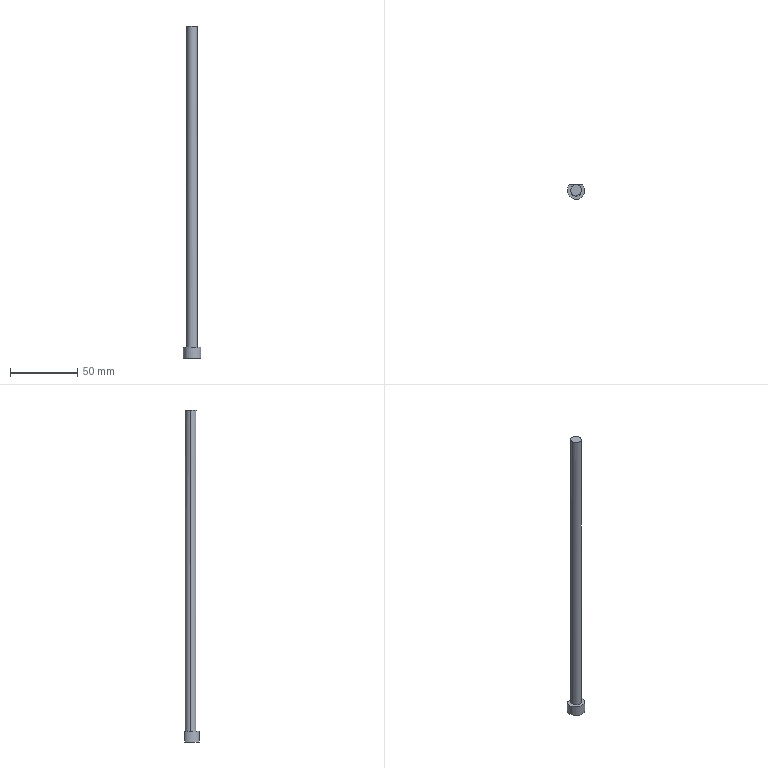Part | Creo | 1 solid | 7 faces | box 13 x 11 x 246.801 mm | volume 12961 mm3 | plane 4 | cylinder 3 | commonest cylinder face diameters 8 x2 13 x1
STEP:
#1=CARTESIAN_POINT('',(0.,0.,0.));
#2=DIRECTION('',(0.,0.,1.));
#3=DIRECTION('',(1.,0.,0.));
#4=AXIS2_PLACEMENT_3D('',#1,#2,#3);
#5=CARTESIAN_POINT('',(94.951,-2.288,-330.441));
#6=VERTEX_POINT('',#5);
#7=CARTESIAN_POINT('',(93.142,-6.788,-330.441));
#8=VERTEX_POINT('',#7);
#9=CARTESIAN_POINT('',(99.642,-6.788,-330.441));
#10=DIRECTION('',(0.,0.,1.));
#11=DIRECTION('',(-0.7216,0.6923,0.));
#12=AXIS2_PLACEMENT_3D('',#9,#10,#11);
#13=CIRCLE('',#12,6.5);
#14=EDGE_CURVE('',#6,#8,#13,.T.);
#15=ORIENTED_EDGE('',*,*,#14,.F.);
#16=CARTESIAN_POINT('',(104.332,-2.288,-330.441));
#17=VERTEX_POINT('',#16);
#18=CARTESIAN_POINT('',(94.951,-2.288,-330.441));
#19=DIRECTION('',(1.,0.,0.));
#20=VECTOR('',#19,9.381);
#21=LINE('',#18,#20);
#22=EDGE_CURVE('',#6,#17,#21,.T.);
#23=ORIENTED_EDGE('',*,*,#22,.T.);
#24=CARTESIAN_POINT('',(99.642,-6.788,-330.441));
#25=DIRECTION('',(0.,0.,1.));
#26=DIRECTION('',(-1.,0.,0.));
#27=AXIS2_PLACEMENT_3D('',#24,#25,#26);
#28=CIRCLE('',#27,6.5);
#29=EDGE_CURVE('',#8,#17,#28,.T.);
#30=ORIENTED_EDGE('',*,*,#29,.F.);
#31=EDGE_LOOP('',(#15,#23,#30));
#32=FACE_OUTER_BOUND('',#31,.F.);
#33=CARTESIAN_POINT('',(103.642,-6.788,-330.441));
#34=VERTEX_POINT('',#33);
#35=CARTESIAN_POINT('',(95.642,-6.788,-330.441));
#36=VERTEX_POINT('',#35);
#37=CARTESIAN_POINT('',(99.642,-6.788,-330.441));
#38=DIRECTION('',(0.,0.,-1.));
#39=DIRECTION('',(1.,0.,0.));
#40=AXIS2_PLACEMENT_3D('',#37,#38,#39);
#41=CIRCLE('',#40,4.);
#42=EDGE_CURVE('',#34,#36,#41,.T.);
#43=ORIENTED_EDGE('',*,*,#42,.F.);
#44=CARTESIAN_POINT('',(99.642,-6.788,-330.441));
#45=DIRECTION('',(0.,0.,-1.));
#46=DIRECTION('',(-1.,0.,0.));
#47=AXIS2_PLACEMENT_3D('',#44,#45,#46);
#48=CIRCLE('',#47,4.);
#49=EDGE_CURVE('',#36,#34,#48,.T.);
#50=ORIENTED_EDGE('',*,*,#49,.F.);
#51=EDGE_LOOP('',(#43,#50));
#52=FACE_BOUND('',#51,.F.);
#53=CARTESIAN_POINT('',(99.642,-6.788,-330.441));
#54=DIRECTION('',(0.,0.,1.));
#55=DIRECTION('',(1.,0.,0.));
#56=AXIS2_PLACEMENT_3D('',#53,#54,#55);
#57=PLANE('',#56);
#58=ADVANCED_FACE('',(#32,#52),#57,.T.);
#59=ORIENTED_EDGE('',*,*,#42,.T.);
#60=CARTESIAN_POINT('',(95.642,-6.786,-91.64));
#61=VERTEX_POINT('',#60);
#62=CARTESIAN_POINT('',(95.642,-6.788,-330.441));
#63=DIRECTION('',(0.000000004,0.000007085,1.));
#64=VECTOR('',#63,238.801);
#65=LINE('',#62,#64);
#66=EDGE_CURVE('',#36,#61,#65,.T.);
#67=ORIENTED_EDGE('',*,*,#66,.T.);
#68=CARTESIAN_POINT('',(103.642,-6.788,-91.651));
#69=VERTEX_POINT('',#68);
#70=CARTESIAN_POINT('',(95.642,-6.786,-91.64));
#71=CARTESIAN_POINT('',(95.642,-7.182,-91.64));
#72=CARTESIAN_POINT('',(95.752,-7.93,-91.641));
#73=CARTESIAN_POINT('',(96.234,-8.986,-91.641));
#74=CARTESIAN_POINT('',(96.983,-9.847,-91.642));
#75=CARTESIAN_POINT('',(97.943,-10.47,-91.643));
#76=CARTESIAN_POINT('',(99.052,-10.8,-91.645));
#77=CARTESIAN_POINT('',(100.2,-10.804,-91.646));
#78=CARTESIAN_POINT('',(101.309,-10.484,-91.648));
#79=CARTESIAN_POINT('',(102.279,-9.867,-91.649));
#80=CARTESIAN_POINT('',(103.042,-9.001,-91.65));
#81=CARTESIAN_POINT('',(103.531,-7.934,-91.651));
#82=CARTESIAN_POINT('',(103.642,-7.182,-91.651));
#83=CARTESIAN_POINT('',(103.642,-6.788,-91.651));
#84=B_SPLINE_CURVE_WITH_KNOTS('',3,(#70,#71,#72,#73,#74,#75,#76,#77,#78,#79,#80,#81,#82,#83),.UNSPECIFIED.,.F.,.F.,(4,1,1,1,1,1,1,1,1,1,1,4),(0.,0.09091,0.1818,0.2727,0.3636,0.4545,0.5455,0.6364,0.7273,0.8182,0.9091,1.),.UNSPECIFIED.);
#85=EDGE_CURVE('',#61,#69,#84,.T.);
#86=ORIENTED_EDGE('',*,*,#85,.T.);
#87=CARTESIAN_POINT('',(103.642,-6.788,-330.441));
#88=DIRECTION('',(0.,0.,1.));
#89=VECTOR('',#88,238.791);
#90=LINE('',#87,#89);
#91=EDGE_CURVE('',#34,#69,#90,.T.);
#92=ORIENTED_EDGE('',*,*,#91,.F.);
#93=EDGE_LOOP('',(#59,#67,#86,#92));
#94=FACE_OUTER_BOUND('',#93,.F.);
#95=CARTESIAN_POINT('',(99.642,-6.788,-653.441));
#96=DIRECTION('',(0.,0.,1.));
#97=DIRECTION('',(1.,0.,0.));
#98=AXIS2_PLACEMENT_3D('',#95,#96,#97);
#99=CYLINDRICAL_SURFACE('',#98,4.);
#100=ADVANCED_FACE('',(#94),#99,.T.);
#101=ORIENTED_EDGE('',*,*,#49,.T.);
#102=ORIENTED_EDGE('',*,*,#91,.T.);
#103=CARTESIAN_POINT('',(103.642,-6.788,-91.651));
#104=CARTESIAN_POINT('',(103.642,-6.395,-91.651));
#105=CARTESIAN_POINT('',(103.531,-5.645,-91.651));
#106=CARTESIAN_POINT('',(103.049,-4.589,-91.65));
#107=CARTESIAN_POINT('',(102.292,-3.72,-91.649));
#108=CARTESIAN_POINT('',(101.323,-3.099,-91.648));
#109=CARTESIAN_POINT('',(100.219,-2.775,-91.646));
#110=CARTESIAN_POINT('',(99.069,-2.774,-91.645));
#111=CARTESIAN_POINT('',(97.965,-3.097,-91.644));
#112=CARTESIAN_POINT('',(96.995,-3.717,-91.642));
#113=CARTESIAN_POINT('',(96.237,-4.585,-91.641));
#114=CARTESIAN_POINT('',(95.754,-5.639,-91.641));
#115=CARTESIAN_POINT('',(95.642,-6.393,-91.64));
#116=CARTESIAN_POINT('',(95.642,-6.786,-91.64));
#117=B_SPLINE_CURVE_WITH_KNOTS('',3,(#103,#104,#105,#106,#107,#108,#109,#110,#111,#112,#113,#114,#115,#116),.UNSPECIFIED.,.F.,.F.,(4,1,1,1,1,1,1,1,1,1,1,4),(0.,0.09091,0.1818,0.2727,0.3636,0.4545,0.5455,0.6364,0.7273,0.8182,0.9091,1.),.UNSPECIFIED.);
#118=EDGE_CURVE('',#69,#61,#117,.T.);
#119=ORIENTED_EDGE('',*,*,#118,.T.);
#120=ORIENTED_EDGE('',*,*,#66,.F.);
#121=EDGE_LOOP('',(#101,#102,#119,#120));
#122=FACE_OUTER_BOUND('',#121,.F.);
#123=CARTESIAN_POINT('',(99.642,-6.788,-653.441));
#124=DIRECTION('',(0.,0.,1.));
#125=DIRECTION('',(1.,0.,0.));
#126=AXIS2_PLACEMENT_3D('',#123,#124,#125);
#127=CYLINDRICAL_SURFACE('',#126,4.);
#128=ADVANCED_FACE('',(#122),#127,.T.);
#129=ORIENTED_EDGE('',*,*,#85,.F.);
#130=ORIENTED_EDGE('',*,*,#118,.F.);
#131=EDGE_LOOP('',(#129,#130));
#132=FACE_OUTER_BOUND('',#131,.F.);
#133=CARTESIAN_POINT('',(248.993,54.022,-91.842));
#134=DIRECTION('',(-0.001312,0.000001665,-1.));
#135=DIRECTION('',(-1.,0.,0.001312));
#136=AXIS2_PLACEMENT_3D('',#133,#134,#135);
#137=PLANE('',#136);
#138=ADVANCED_FACE('',(#132),#137,.F.);
#139=CARTESIAN_POINT('',(104.332,-2.288,-338.441));
#140=VERTEX_POINT('',#139);
#141=CARTESIAN_POINT('',(104.332,-2.288,-338.441));
#142=DIRECTION('',(0.,0.,1.));
#143=VECTOR('',#142,8.);
#144=LINE('',#141,#143);
#145=EDGE_CURVE('',#140,#17,#144,.T.);
#146=ORIENTED_EDGE('',*,*,#145,.F.);
#147=CARTESIAN_POINT('',(93.142,-6.788,-338.441));
#148=VERTEX_POINT('',#147);
#149=CARTESIAN_POINT('',(99.642,-6.788,-338.441));
#150=DIRECTION('',(0.,0.,-1.));
#151=DIRECTION('',(0.7216,0.6923,0.));
#152=AXIS2_PLACEMENT_3D('',#149,#150,#151);
#153=CIRCLE('',#152,6.5);
#154=EDGE_CURVE('',#140,#148,#153,.T.);
#155=ORIENTED_EDGE('',*,*,#154,.T.);
#156=CARTESIAN_POINT('',(94.951,-2.288,-338.441));
#157=VERTEX_POINT('',#156);
#158=CARTESIAN_POINT('',(99.642,-6.788,-338.441));
#159=DIRECTION('',(0.,0.,-1.));
#160=DIRECTION('',(-1.,0.,0.));
#161=AXIS2_PLACEMENT_3D('',#158,#159,#160);
#162=CIRCLE('',#161,6.5);
#163=EDGE_CURVE('',#148,#157,#162,.T.);
#164=ORIENTED_EDGE('',*,*,#163,.T.);
#165=CARTESIAN_POINT('',(94.951,-2.288,-330.441));
#166=DIRECTION('',(0.,0.,-1.));
#167=VECTOR('',#166,8.);
#168=LINE('',#165,#167);
#169=EDGE_CURVE('',#6,#157,#168,.T.);
#170=ORIENTED_EDGE('',*,*,#169,.F.);
#171=ORIENTED_EDGE('',*,*,#14,.T.);
#172=ORIENTED_EDGE('',*,*,#29,.T.);
#173=EDGE_LOOP('',(#146,#155,#164,#170,#171,#172));
#174=FACE_OUTER_BOUND('',#173,.F.);
#175=CARTESIAN_POINT('',(99.642,-6.788,-330.441));
#176=DIRECTION('',(0.,0.,-1.));
#177=DIRECTION('',(-1.,0.,0.));
#178=AXIS2_PLACEMENT_3D('',#175,#176,#177);
#179=CYLINDRICAL_SURFACE('',#178,6.5);
#180=ADVANCED_FACE('',(#174),#179,.T.);
#181=ORIENTED_EDGE('',*,*,#22,.F.);
#182=ORIENTED_EDGE('',*,*,#169,.T.);
#183=CARTESIAN_POINT('',(94.951,-2.288,-338.441));
#184=DIRECTION('',(1.,0.,0.));
#185=VECTOR('',#184,9.381);
#186=LINE('',#183,#185);
#187=EDGE_CURVE('',#157,#140,#186,.T.);
#188=ORIENTED_EDGE('',*,*,#187,.T.);
#189=ORIENTED_EDGE('',*,*,#145,.T.);
#190=EDGE_LOOP('',(#181,#182,#188,#189));
#191=FACE_OUTER_BOUND('',#190,.F.);
#192=CARTESIAN_POINT('',(99.642,-2.288,-338.441));
#193=DIRECTION('',(0.,1.,0.));
#194=DIRECTION('',(0.,0.,1.));
#195=AXIS2_PLACEMENT_3D('',#192,#193,#194);
#196=PLANE('',#195);
#197=ADVANCED_FACE('',(#191),#196,.T.);
#198=ORIENTED_EDGE('',*,*,#187,.F.);
#199=ORIENTED_EDGE('',*,*,#163,.F.);
#200=ORIENTED_EDGE('',*,*,#154,.F.);
#201=EDGE_LOOP('',(#198,#199,#200));
#202=FACE_OUTER_BOUND('',#201,.F.);
#203=CARTESIAN_POINT('',(99.642,-6.788,-338.441));
#204=DIRECTION('',(0.,0.,1.));
#205=DIRECTION('',(1.,0.,0.));
#206=AXIS2_PLACEMENT_3D('',#203,#204,#205);
#207=PLANE('',#206);
#208=ADVANCED_FACE('',(#202),#207,.F.);
#209=CLOSED_SHELL('',(#58,#100,#128,#138,#180,#197,#208));
#210=MANIFOLD_SOLID_BREP('',#209);
#211=(LENGTH_UNIT()NAMED_UNIT(*)SI_UNIT(.MILLI.,.METRE.));
#212=UNCERTAINTY_MEASURE_WITH_UNIT(LENGTH_MEASURE(0.02474),#211,'','');
#213=(NAMED_UNIT(*)PLANE_ANGLE_UNIT()SI_UNIT($,.RADIAN.));
#214=PLANE_ANGLE_MEASURE_WITH_UNIT(PLANE_ANGLE_MEASURE(0.01745),#213);
#215=(CONVERSION_BASED_UNIT('DEGREE',#214)NAMED_UNIT(*)PLANE_ANGLE_UNIT());
#216=(NAMED_UNIT(*)SI_UNIT($,.STERADIAN.)SOLID_ANGLE_UNIT());
#217=(GEOMETRIC_REPRESENTATION_CONTEXT(3)GLOBAL_UNCERTAINTY_ASSIGNED_CONTEXT((#212))GLOBAL_UNIT_ASSIGNED_CONTEXT((#211,#215,#216))REPRESENTATION_CONTEXT('',''));
#218=ADVANCED_BREP_SHAPE_REPRESENTATION('',(#4,#210),#217);